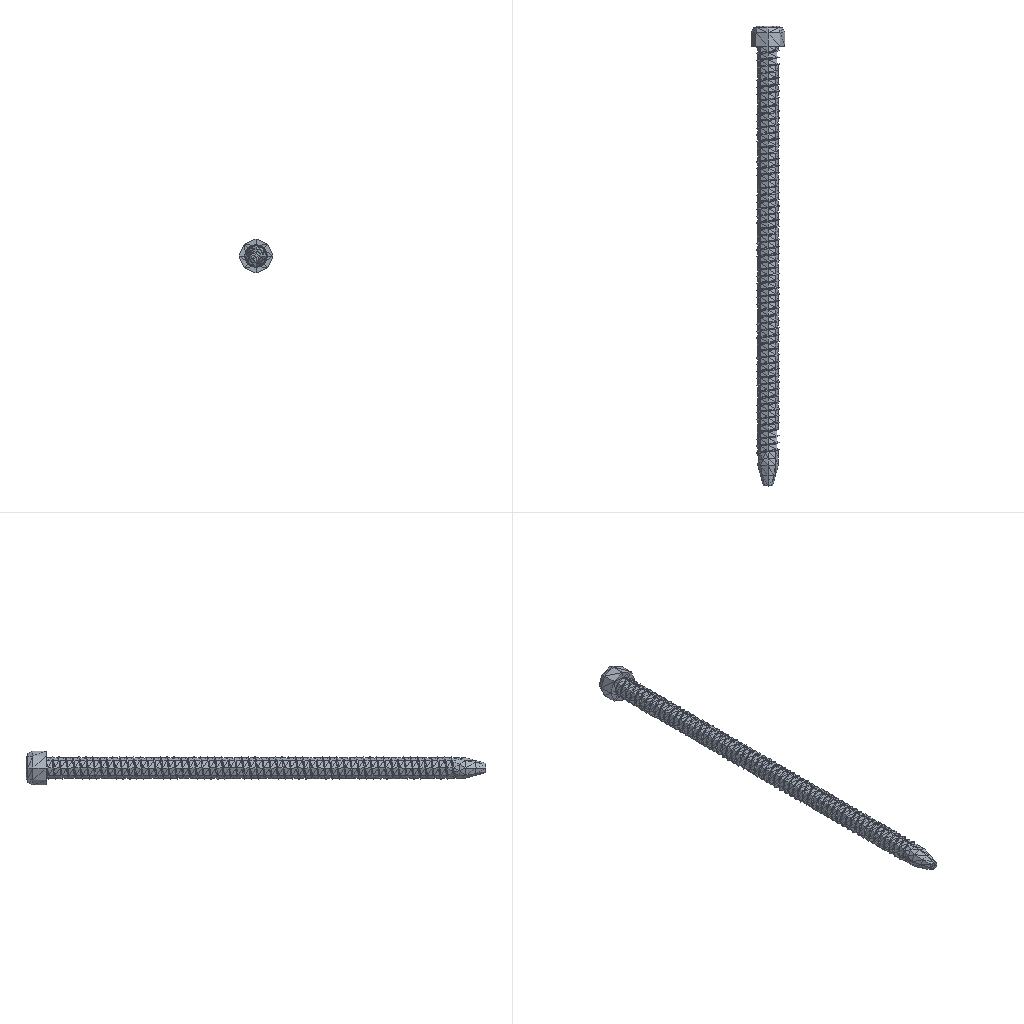Simulation study | abaqus
Set-up summary:
category,name,step,type,value,unit,region
solver,abaqus
solver,version,,,Abaqus/Standard 2022
units,not stated in the deck,,not stated
analysis,deck,,static,static
load_step,Step-1,Step-1,static,nlgeom=False
contact,interactions,,,general=0 pairs=0 ties=0
load_step,requested,,,1
mesh,nodes,,,17629
mesh,elements,,,9559
element_type,C3D10,,solid,9559
load,load commands in deck,,count,1
bc,support commands in deck,,count,1
material,MATERIAL-1,,in results
check,setup vs results,,match,"per instance, exact: element labels, types and connectivity; labels of the nodes the elements use; coordinates of those nodes at SINGLE_PRECISION in 1 of 1 instance(s)"
Results summary:
result,step,,partial,increments=0 time=0.0/1.0
result,analysis,,,static
result,last_loadstep,,,1
result,analysis steps,,count,1
result,primary field,,,U
result,reaction total,,FX,4e-06,model units
result,reaction total,,FY,1500,model units
result,reaction total,,FZ,1e-06,model units